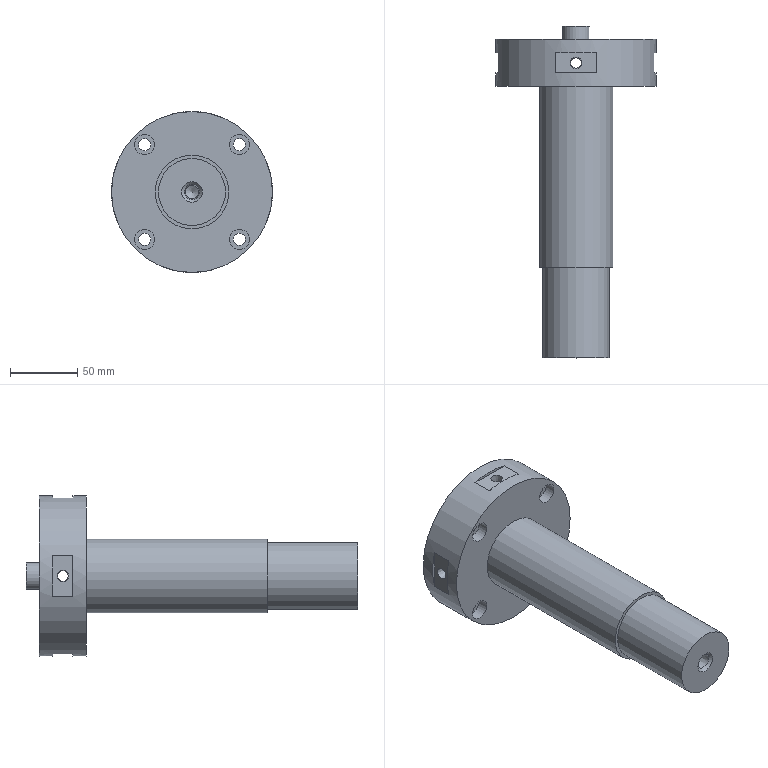Part | STEP file | Part [22] | 1 solid | 71 faces | box 120 x 247.5 x 120 mm | volume 802032 mm3 | cylinder 34 | plane 25 | cone 12 | commonest cylinder face diameters 8 x16 15 x8 9 x4 10 x2 20 x1 50 x1